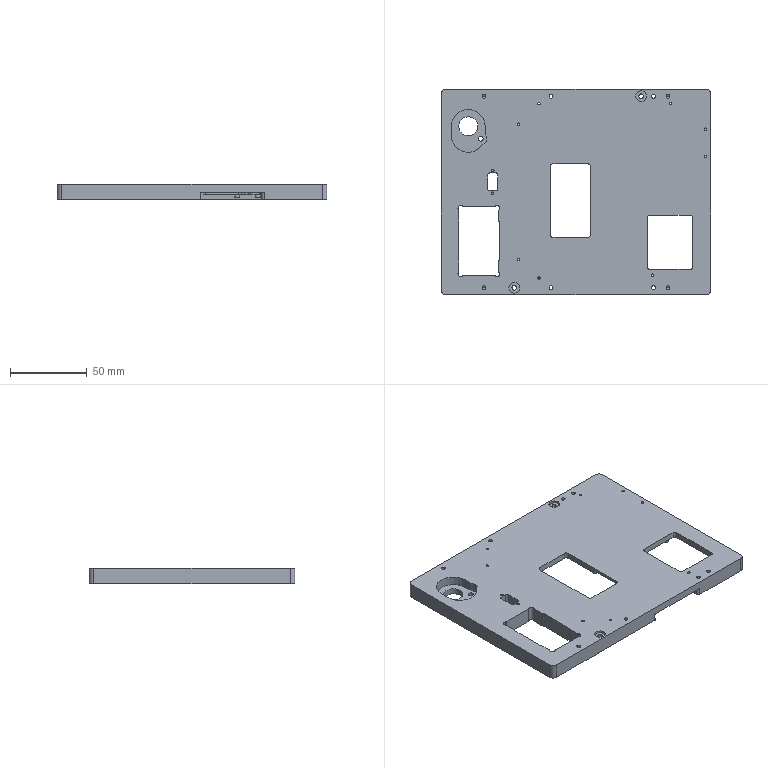NC program | NX | posted with a generic post | part box 176 x 134 x 10 mm
Lines 98 to 1138 of 17594:
(CAVITY_MILL , TOOL : D10)
N188 T04 M6
N190 G54
N192 G17 G0 G90 X-20.503 Y3.162 S9500 M3
N194 G43 Z30. H4
N196 Z1.5
N198 G94 G1 Y4.346 Z1.438 F1000.
N200 X-22.187 Y3.255 Z1.333
N202 X-22.361 Y3.15 Z1.322
N204 X-25.859 Y1.182 Z1.112
N206 X-26.039 Y1.088 Z1.101
N208 X-27.847 Y0.216 Z0.996
N210 X-26.039 Y-0.656 Z0.891
N212 X-22.187 Y-2.823 Z0.659
N214 X-20.503 Y-3.914 Z0.554
N216 Y4.346 Z0.121
N218 X-22.187 Y3.255 Z0.016
N220 X-22.361 Y3.15 Z0.005
N222 X-24.11 Y2.166 Z-0.1
N224 G2 X-27.847 Y0.216 R67.1 F3000.
N226 X-20.503 Y-3.914 R67.1
N228 G1 Y4.346
N230 G2 X-24.11 Y2.166 R67.1
N232 G1 X-26.316 Y6.088
N234 G2 X-32.497 Y3.047 R62.6
N236 G1 Y-2.614
N238 G2 X-17.697 Y-11.497 R62.6
N240 G1 X-16.003
N242 Y11.497
N244 X-18.239
N246 G2 X-26.316 Y6.088 R62.6
N248 G1 X-29.747 Y12.189
N250 G2 X-39.497 Y7.878 R55.6
N252 G1 Y-7.446
N254 G2 X-20.252 Y-18.497 R55.6
N256 G1 X-9.003
N258 Y18.497
N260 X-20.748
N262 G2 X-29.747 Y12.189 R55.6
N264 G1 X-33.179 Y18.291
N266 G2 X-46.497 Y13.2 R48.6
N268 G1 Y-12.768
N270 G2 X-22.998 Y-25.497 R48.6
N272 G1 X-2.003
N274 Y25.497
N276 X-23.444
N278 G2 X-33.179 Y18.291 R48.6
N280 G1 X-36.61 Y24.392
N282 G2 X-53.497 Y19.199 R41.6
N284 G1 Y-16.474
N286 G2 X-50.323 Y-19.158 R41.6
N288 X-25.986 Y-32.497 R41.6
N290 G1 X4.997
N292 Y32.497
N294 X-26.377
N296 G2 X-36.61 Y24.392 R41.6
N298 G1 X-40.042 Y30.493
N300 G2 X-57.003 Y26.051 R34.6
N302 G1 X-58.134
N304 G2 X-60.497 Y26.135 R33.1
N306 G1 Y-20.141
N308 G2 X-53.579 Y-25.788 R34.6
N310 X-29.294 Y-39.497 R34.6
N312 G1 X11.997
N314 Y39.497
N316 X-29.623
N318 G2 X-40.042 Y30.493 R34.6
N320 G1 X-43.473 Y36.594
N322 G2 X-57.003 Y33.051 R27.6
N324 G1 X-58.134
N326 G2 X-62.194 Y33.368 R26.1
N328 X-63.881 Y33.163 R27.6
N330 X-67.497 Y31.216 R27.6
N332 G1 Y-24.335
N334 G2 X-56.935 Y-32.619 R27.6
N336 X-33.055 Y-46.497 R27.6
N338 G1 X18.997
N340 Y46.497
N342 X-33.308
N344 G2 X-43.473 Y36.594 R27.6
N346 G1 X-46.904 Y42.695
N348 G2 X-57.003 Y40.051 R20.6
N350 G1 X-58.134
N352 G2 X-62.173 Y40.483 R19.1
N354 X-66.235 Y40.051 R20.6
N356 X-74.497 Y36.265 R20.6
N358 G1 Y-29.384
N360 G2 X-60.685 Y-39.619 R20.6
N362 G1 X-57.003
N364 G2 X-37.53 Y-53.497 R20.6
N366 G1 X25.997
N368 Y53.497
N370 X-37.685
N372 G2 X-46.904 Y42.695 R20.6
N374 G1 X-50.336 Y48.797
N376 G2 X-57.003 Y47.051 R13.6
N378 G1 X-58.134
N380 G2 X-62.128 Y47.729 R12.1
N382 X-66.37 Y47.051 R13.6
N384 G1 X-68.883
N386 G2 X-78.737 Y42.824 R13.6
N388 G1 X-81.497
N390 Y-35.943
N392 X-78.737
N394 G2 X-65.455 Y-46.619 R13.6
N396 G1 X-57.003
N398 G2 X-43.403 Y-60.219 R13.6
N400 G1 Y-60.497
N402 X32.997
N404 Y60.497
N406 X-43.404
N408 G2 X-50.336 Y48.797 R13.6
N410 G1 X-53.767 Y54.898
N412 G2 X-57.003 Y54.051 R6.6
N414 G1 X-58.134
N416 G2 X-61.941 Y55.757 R5.1
N418 X-66.37 Y54.051 R6.6
N420 G1 X-72.578
N422 G2 X-78.737 Y49.824 R6.6
N424 G1 X-86.5
N426 G2 X-92.997 Y55.262 R6.6
N428 G1 Y51.756
N430 G3 X-88.497 Y48.677 R8.
N432 G1 Y-41.796
N434 G3 X-92.997 Y-44.875 R8.
N436 G1 Y-48.38
N438 G2 X-86.5 Y-42.943 R6.6
N440 G1 X-78.737
N442 G2 X-72.137 Y-49.543 R6.6
N444 G1 Y-53.619
N446 X-57.003
N448 G2 X-50.403 Y-60.219 R6.6
N450 G1 Y-64.258
N452 G2 X-55.722 Y-71.997 R6.6
N454 G1 X-52.216
N456 G3 X-49.138 Y-67.497 R8.
N458 G1 X38.733
N460 G3 X41.811 Y-71.997 R8.
N462 G1 X45.316
N464 G2 X39.997 Y-64.258 R6.6
N466 G1 Y64.258
N468 G2 X45.316 Y71.997 R6.6
N470 G1 X41.811
N472 G3 X38.733 Y67.497 R8.
N474 G1 X-49.138
N476 G3 X-52.216 Y71.997 R8.
N478 G1 X-55.722
N480 G2 X-50.403 Y64.258 R6.6
N482 G1 Y60.576
N484 G2 X-53.767 Y54.898 R6.6
N486 G3 X-54.277 Y54.038 R1.
N488 G1 Z1.4
N490 G0 Z30.
N492 X-30.878 Y0.551
N494 Z1.4
N496 G1 X-34.997 Z1.184 F1000.
N498 Y-1.364 Z1.084
N500 X-33.137 Y-1.748 Z0.984
N502 X-28.184 Y-3.164 Z0.714
N504 X-26.402 Y-3.82 Z0.615
N506 X-24.62 Y-3.164 Z0.515
N508 X-21.303 Y-2.165 Z0.334
N510 X-19.454 Y-1.728 Z0.234
N512 Y0.551 Z0.115
N514 X-34.997 Z-0.7
N516 Y-0.406 Z-0.75
N518 Y-1.364 F3000.
N520 G2 X-26.402 Y-3.82 R60.1
N522 X-19.454 Y-1.728 R60.1
N524 G1 Y0.551
N526 X-34.997
N528 Y-0.406
N530 X-39.497
N532 Y-5.15
N534 G2 X-26.402 Y-8.642 R55.6
N536 X-14.954 Y-5.405 R55.6
N538 G1 Y5.051
N540 X-39.497
N542 Y-0.406
N544 X-46.497
N546 Y-11.623
N548 G2 X-26.402 Y-16.278 R48.6
N550 X-7.954 Y-11.674 R48.6
N552 G1 Y12.051
N554 X-46.497
N556 Y-0.406
N558 X-53.497
N560 Y-16.474
N562 G2 X-50.911 Y-18.619 R41.6
N564 G1 X-47.167
N566 G2 X-26.402 Y-24.172 R41.6
N568 X-5.63 Y-18.619 R41.6
N570 G1 X-0.954
N572 Y19.051
N574 X-53.497
N576 Y-0.406
N578 X-60.497
N580 Y-20.141
N582 G2 X-53.741 Y-25.619 R34.6
N584 G1 X-47.167
N586 G2 X-26.402 Y-32.542 R34.6
N588 X-5.631 Y-25.619 R34.6
N590 G1 X6.046
N592 Y26.051
N594 X-58.134
N596 G2 X-60.497 Y26.135 R33.1
N598 G1 Y-0.406
N600 X-67.497
N602 Y-24.335
N604 G2 X-56.935 Y-32.619 R27.6
N606 G1 X-47.167
N608 G2 X-26.402 Y-42.037 R27.6
N610 X-5.632 Y-32.619 R27.6
N612 G1 X13.046
N614 Y33.051
N616 X-58.134
N618 G2 X-62.194 Y33.368 R26.1
N620 X-63.881 Y33.163 R27.6
N622 X-67.497 Y31.216 R27.6
N624 G1 Y-0.406
N626 X-74.497
N628 Y-29.384
N630 G2 X-60.685 Y-39.619 R20.6
N632 G1 X-47.167
N634 G2 X-27.694 Y-53.497 R20.6
N636 G1 X-25.109
N638 G2 X-5.633 Y-39.619 R20.6
N640 G1 X20.046
N642 X20.045 Y39.689
N644 G2 X20.049 Y40.056 R20.6
N646 X19.588 Y40.051 R20.6
N648 G1 X-58.134
N650 G2 X-62.173 Y40.483 R19.1
N652 X-66.235 Y40.051 R20.6
N654 X-74.497 Y36.265 R20.6
N656 G1 Y-0.406
N658 X-81.497
N660 Y-35.943
N662 X-78.737
N664 G2 X-65.455 Y-46.619 R13.6
N666 G1 X-47.167
N668 G2 X-33.567 Y-60.219 R13.6
N670 G1 Y-60.497
N672 X-19.234
N674 G2 X-5.634 Y-46.619 R13.6
N676 G1 X20.441
N678 G2 X24.201 Y-47.149 R13.6
N680 X27.175 Y-46.641 R13.6
N682 X27.816 Y-44. R13.6
N684 X27.045 Y-39.488 R13.6
N686 G1 Y39.689
N688 G2 X27.834 Y44.253 R13.6
N690 X27.148 Y47.153 R13.6
N692 X24.201 Y47.857 R13.6
N694 X19.588 Y47.051 R13.6
N696 G1 X-58.134
N698 G2 X-62.128 Y47.729 R12.1
N700 X-66.37 Y47.051 R13.6
N702 G1 X-68.883
N704 G2 X-78.737 Y42.824 R13.6
N706 G1 X-81.497
N708 Y-0.406
N710 X-88.497
N712 Y-41.796
N714 G3 X-92.997 Y-44.875 R8.
N716 G1 Y-48.381
N718 G2 X-86.5 Y-42.943 R6.6
N720 G1 X-78.737
N722 G2 X-72.137 Y-49.543 R6.6
N724 G1 Y-53.619
N726 X-47.167
N728 G2 X-40.567 Y-60.219 R6.6
N730 G1 Y-65.5
N732 G2 X-46.005 Y-71.997 R6.6
N734 G1 X-42.499
N736 G3 X-39.42 Y-67.497 R8.
N738 G1 X-13.381
N740 G3 X-10.302 Y-71.997 R8.
N742 G1 X-6.796
N744 G2 X-12.234 Y-65.5 R6.6
N746 G1 Y-60.219
N748 G2 X-5.634 Y-53.619 R6.6
N750 G1 X20.441
N752 G2 X24.201 Y-54.794 R6.6
N754 X27.961 Y-53.619 R6.6
N756 G1 X34.045
N758 Y-48.512
N760 G2 X35.828 Y-44. R6.6
N762 X34.045 Y-39.488 R6.6
N764 G1 Y39.689
N766 G2 X35.878 Y44.253 R6.6
N768 X34.045 Y48.817 R6.6
N770 G1 Y54.051
N772 X28.814
N774 G2 X24.338 Y55.8 R6.6
N776 G1 X24.2 Y55.93
N778 G2 X19.588 Y54.051 R6.6
N780 G1 X-58.134
N782 G2 X-61.941 Y55.757 R5.1
N784 X-66.37 Y54.051 R6.6
N786 G1 X-72.578
N788 G2 X-78.737 Y49.824 R6.6
N790 G1 X-86.5
N792 G2 X-92.997 Y55.263 R6.6
N794 G1 Y51.756
N796 G3 X-88.497 Y48.677 R8.
N798 G1 Y-0.406
N800 G2 X-88.997 Y-1.273 R1.
N802 G1 X-94.997 Y-4.737
N804 Z0.75
N806 G0 Z30.
N808 X-30.878 Y0.551
N810 Z0.75
N812 G1 X-34.997 Z0.534 F1000.
N814 Y-1.364 Z0.434
N816 X-33.137 Y-1.748 Z0.334
N818 X-28.184 Y-3.164 Z0.064
N820 X-26.402 Y-3.82 Z-0.035
N822 X-24.62 Y-3.164 Z-0.135
N824 X-21.303 Y-2.165 Z-0.316
N826 X-19.454 Y-1.728 Z-0.416
N828 Y0.551 Z-0.535
N830 X-34.997 Z-1.35
N832 Y-0.406 Z-1.4
N834 Y-1.364 F3000.
N836 G2 X-26.402 Y-3.82 R60.1
N838 X-19.454 Y-1.728 R60.1
N840 G1 Y0.551
N842 X-34.997
N844 Y-0.406
N846 X-39.497
N848 Y-5.15
N850 G2 X-26.402 Y-8.642 R55.6
N852 X-14.954 Y-5.405 R55.6
N854 G1 Y5.051
N856 X-39.497
N858 Y-0.406
N860 X-46.497
N862 Y-11.623
N864 G2 X-26.402 Y-16.278 R48.6
N866 X-7.954 Y-11.674 R48.6
N868 G1 Y12.051
N870 X-46.497
N872 Y-0.406
N874 X-53.497
N876 Y-16.474
N878 G2 X-50.911 Y-18.619 R41.6
N880 G1 X-47.167
N882 G2 X-26.402 Y-24.172 R41.6
N884 X-5.631 Y-18.619 R41.6
N886 G1 X-0.954
N888 Y19.051
N890 X-53.497
N892 Y-0.406
N894 X-60.497
N896 Y-20.141
N898 G2 X-53.741 Y-25.619 R34.6
N900 G1 X-47.167
N902 G2 X-26.402 Y-32.542 R34.6
N904 X-5.631 Y-25.619 R34.6
N906 G1 X6.046
N908 Y26.051
N910 X-58.134
N912 G2 X-60.497 Y26.135 R33.1
N914 G1 Y-0.406
N916 X-67.497
N918 Y-24.335
N920 G2 X-56.935 Y-32.619 R27.6
N922 G1 X-47.167
N924 G2 X-26.402 Y-42.037 R27.6
N926 X-5.632 Y-32.619 R27.6
N928 G1 X13.046
N930 Y33.051
N932 X-58.134
N934 G2 X-62.194 Y33.368 R26.1
N936 X-63.881 Y33.163 R27.6
N938 X-67.497 Y31.216 R27.6
N940 G1 Y-0.406
N942 X-74.497
N944 Y-29.384
N946 G2 X-60.685 Y-39.619 R20.6
N948 G1 X-47.167
N950 G2 X-27.694 Y-53.497 R20.6
N952 G1 X-25.109
N954 G2 X-5.633 Y-39.619 R20.6
N956 G1 X20.046
N958 X20.045 Y39.689
N960 G2 X20.049 Y40.056 R20.6
N962 X19.588 Y40.051 R20.6
N964 G1 X-58.134
N966 G2 X-62.173 Y40.483 R19.1
N968 X-66.235 Y40.051 R20.6
N970 X-74.497 Y36.265 R20.6
N972 G1 Y-0.406
N974 X-81.497
N976 Y-35.943
N978 X-78.737
N980 G2 X-65.455 Y-46.619 R13.6
N982 G1 X-47.167
N984 G2 X-33.567 Y-60.219 R13.6
N986 G1 Y-60.497
N988 X-19.234
N990 G2 X-5.634 Y-46.619 R13.6
N992 G1 X20.441
N994 G2 X24.201 Y-47.149 R13.6
N996 X27.175 Y-46.641 R13.6
N998 X27.816 Y-44. R13.6
N1000 X27.045 Y-39.488 R13.6
N1002 G1 Y39.689
N1004 G2 X27.834 Y44.253 R13.6
N1006 X27.148 Y47.153 R13.6
N1008 X24.201 Y47.857 R13.6
N1010 X19.588 Y47.051 R13.6
N1012 G1 X-58.134
N1014 G2 X-62.128 Y47.729 R12.1
N1016 X-66.37 Y47.051 R13.6
N1018 G1 X-68.883
N1020 G2 X-78.737 Y42.824 R13.6
N1022 G1 X-81.497
N1024 Y-0.406
N1026 X-88.497
N1028 Y-41.796
N1030 G3 X-92.997 Y-44.875 R8.
N1032 G1 Y-48.382
N1034 G2 X-86.5 Y-42.943 R6.6
N1036 G1 X-78.737
N1038 G2 X-72.137 Y-49.543 R6.6
N1040 G1 Y-53.619
N1042 X-47.167
N1044 G2 X-40.567 Y-60.219 R6.6
N1046 G1 Y-65.5
N1048 G2 X-46.006 Y-71.997 R6.6
N1050 G1 X-42.499
N1052 G3 X-39.42 Y-67.497 R8.
N1054 G1 X-13.381
N1056 G3 X-10.302 Y-71.997 R8.
N1058 G1 X-6.795
N1060 G2 X-12.234 Y-65.5 R6.6
N1062 G1 Y-60.219
N1064 G2 X-5.634 Y-53.619 R6.6
N1066 G1 X20.441
N1068 G2 X24.201 Y-54.794 R6.6
N1070 X27.961 Y-53.619 R6.6
N1072 G1 X34.045
N1074 Y-48.512
N1076 G2 X35.828 Y-44. R6.6
N1078 X34.045 Y-39.488 R6.6
N1080 G1 Y39.689
N1082 G2 X35.878 Y44.253 R6.6
N1084 X34.045 Y48.817 R6.6
N1086 G1 Y54.051
N1088 X28.814
N1090 G2 X24.338 Y55.8 R6.6
N1092 G1 X24.2 Y55.93
N1094 G2 X19.588 Y54.051 R6.6
N1096 G1 X-58.134
N1098 G2 X-61.941 Y55.757 R5.1
N1100 X-66.37 Y54.051 R6.6
N1102 G1 X-72.578
N1104 G2 X-78.737 Y49.824 R6.6
N1106 G1 X-86.5
N1108 G2 X-92.997 Y55.264 R6.6
N1110 G1 Y51.756
N1112 G3 X-88.497 Y48.677 R8.
N1114 G1 Y-0.406
N1116 G2 X-88.997 Y-1.273 R1.
N1118 G1 X-94.997 Y-4.737
N1120 Z0.1
N1122 G0 Z30.
N1124 X-24.7 Y-1.606
N1126 Z0.1
N1128 G1 X-24.433 Y-0.962 Z0.063 F1000.
N1130 X-22.568 Y2.7 Z-0.152
N1132 X-20.395 Y6.188 Z-0.367
N1134 X-19.39 Y7.551 Z-0.456
N1136 X-23.62 Z-0.678
N1138 X-23.846 Y6.485 Z-0.735
N1140 X-24.805 Y3.754 Z-0.886
N1142 X-26.151 Y1.191 Z-1.038
N1144 X-27.403 Y-0.592 Z-1.152
N1146 X-28.217 Y-1.56 Z-1.219
N1148 X-28.988 Y-2.33 Z-1.276
N1150 X-27.298 Y-2.345 Z-1.364
N1152 X-26.764 Y-2.372 Z-1.392
N1154 X-25.081 Y-2.526 Z-1.481
N1156 X-24.433 Y-0.962 Z-1.57
N1158 X-22.568 Y2.7 Z-1.785
N1160 X-20.395 Y6.188 Z-2.
N1162 X-19.39 Y7.551 Z-2.089
N1164 X-21.505 Z-2.2
N1166 X-23.62 F3000.
N1168 G2 X-28.988 Y-2.33 R19.76
N1170 X-25.081 Y-2.526 R47.61
N1172 X-19.39 Y7.551 R47.76
N1174 G1 X-21.505
N1176 Y12.051
N1178 X-27.695
N1180 G2 X-46.497 Y-3.188 R15.26
N1182 G1 Y-10.352
N1184 G2 X-22.105 Y-7.454 R43.11
N1186 X-9.102 Y12.051 R43.26
N1188 G1 X-21.505
N1190 Y19.051
N1192 X-39.273
N1194 G2 X-46.626 Y19.051 R-8.26
N1196 G1 X-46.003 Y17.797
N1198 G2 X-36.806 Y14.707 R6.86
N1200 X-46.003 Y17.797 R-6.86
N1202 G1 X-46.626 Y19.051
N1204 X-53.497
N1206 Y-16.474
N1208 G2 X-50.911 Y-18.619 R41.6
N1210 G1 X-47.4
N1212 G2 X-16.905 Y-16.068 R36.11
N1214 X-0.955 Y9.445 R36.26
N1216 G1 Y19.051
N1218 X-21.505
N1220 Y26.051
N1222 X-60.497
N1224 Y-20.14
N1226 G2 X-53.741 Y-25.619 R34.6
N1228 G1 X-47.167
N1230 G2 X-45.487 Y-25.659 R34.6
N1232 X-13.719 Y-25.43 R29.11
N1234 X-10.153 Y-22.715 R34.71
N1236 X6.045 Y5.413 R29.26
N1238 G1 Y26.051
N1240 X-21.505
N1242 Y33.051
N1244 X-60.76
N1246 G2 X-61.81 Y33.071 R27.6
N1248 X-62.86 Y33.051 R27.6
N1250 G1 X-64.058
N1252 G2 X-67.497 Y31.216 R27.6
N1254 G1 Y-24.335
N1256 G2 X-56.935 Y-32.619 R27.6
N1258 G1 X-47.167
N1260 G2 X-43.477 Y-32.866 R27.6
N1262 X-14.141 Y-33.962 R22.11
N1264 X-11.734 Y-33.301 R27.6
N1266 X-2.49 Y-26.437 R27.71
N1268 X13.045 Y0.635 R22.26
N1270 G1 Y33.051
N1272 X-21.505
N1274 Y40.051
N1276 X-60.76
N1278 G2 X-61.81 Y40.077 R20.6
N1280 X-62.86 Y40.051 R20.6
N1282 G1 X-66.236
N1284 G2 X-74.497 Y36.265 R20.6
N1286 G1 Y-29.384
N1288 G2 X-60.685 Y-39.619 R20.6
N1290 G1 X-47.167
N1292 G2 X-41.222 Y-40.495 R20.6
N1294 X-16.241 Y-42.559 R15.11
N1296 X-7.913 Y-39.745 R20.6
N1298 X7.665 Y-30.968 R20.71
N1300 G1 X12.478 Y-32.321
N1302 G3 X22.045 Y-33.717 R13.26
N1304 G1 Y-38.175
N1306 G3 X12.148 Y-33.181 R18.71
N1308 X12.478 Y-32.321 R5.
N1310 G1 X7.665 Y-30.968
N1312 G2 X20.045 Y-5.574 R15.26
N1314 G1 Y40.051
N1316 X-21.505
N1318 Y47.051
N1320 X-60.76
N1322 G2 X-61.81 Y47.091 R13.6
N1324 X-62.86 Y47.051 R13.6
N1326 G1 X-68.883
N1328 G2 X-78.737 Y42.824 R13.6
N1330 G1 X-81.497
N1332 Y-35.943
N1334 X-78.737
N1336 G2 X-65.455 Y-46.619 R13.6
N1338 G1 X-47.167
N1340 G2 X-37.506 Y-50.647 R13.6
N1342 X-34.059 Y-56.595 R-8.11
N1344 G1 X-33.259 Y-55.446
N1346 G2 X-34.934 Y-46.105 R6.71
N1348 X-33.259 Y-55.446 R-6.71
N1350 G1 X-34.059 Y-56.595
N1352 G2 X-33.567 Y-60.219 R13.6
N1354 G1 Y-60.497
N1356 X-19.234
N1358 G2 X-15.251 Y-50.602 R13.6
N1360 X-5.634 Y-46.619 R13.6
N1362 G1 X-3.714
N1364 G2 X21.807 Y-46.619 R13.71
N1366 G1 X27.045
N1368 Y-22.853
N1370 G2 X27.045 Y-18.749 R-8.26
N1372 G1 X25.689 Y-19.097
N1374 G2 X20.749 Y-27.446 R6.86
N1376 X25.689 Y-19.097 R-6.86
N1378 G1 X27.045 Y-18.749
N1380 Y47.051
N1382 X25.464
N1384 G2 X24.201 Y47.109 R13.6
N1386 X22.938 Y47.051 R13.6
N1388 G1 X-21.505
N1390 Y54.051
N1392 X-60.76
N1394 G2 X-61.81 Y54.135 R6.6
N1396 X-62.86 Y54.051 R6.6
N1398 G1 X-72.578
N1400 G2 X-78.737 Y49.824 R6.6
N1402 G1 X-86.5
N1404 G2 X-92.997 Y55.265 R6.6
N1406 G1 Y51.757
N1408 G3 X-88.497 Y48.677 R8.
N1410 G1 Y-41.796
N1412 G3 X-92.997 Y-44.875 R8.
N1414 G1 Y-48.384
N1416 G2 X-86.5 Y-42.943 R6.6
N1418 G1 X-78.737
N1420 G2 X-72.137 Y-49.543 R6.6
N1422 G1 Y-53.619
N1424 X-47.167
N1426 G2 X-40.567 Y-60.219 R6.6
N1428 G1 Y-65.5
N1430 G2 X-46.007 Y-71.997 R6.6
N1432 G1 X-42.499
N1434 G3 X-39.42 Y-67.497 R8.
N1436 G1 X-13.381
N1438 G3 X-10.301 Y-71.997 R8.
N1440 G1 X-6.794
N1442 G2 X-12.234 Y-65.5 R6.6
N1444 G1 Y-60.219
N1446 G2 X-5.634 Y-53.619 R6.6
N1448 G1 X1.183
N1450 X2.637
N1452 G2 X15.455 Y-53.619 R-6.71
N1454 G1 X16.909
N1456 X34.045
N1458 Y54.051
N1460 X25.464
N1462 G2 X24.201 Y54.173 R6.6
N1464 X22.938 Y54.051 R6.6
N1466 G1 X-21.505
N1468 G3 X-22.371 Y53.551 R1.
N1470 G1 Z-0.7
N1472 G0 X-24.7 Y-1.606
N1474 G1 X-24.433 Y-0.962 Z-0.737 F1000.
N1476 X-22.568 Y2.7 Z-0.952
N1478 X-20.395 Y6.188 Z-1.167
N1480 X-19.39 Y7.551 Z-1.256
N1482 X-23.62 Z-1.478
N1484 X-23.846 Y6.485 Z-1.535
N1486 X-24.805 Y3.754 Z-1.686
N1488 X-26.151 Y1.191 Z-1.838
N1490 X-27.403 Y-0.592 Z-1.952
N1492 X-28.217 Y-1.56 Z-2.019
N1494 X-28.988 Y-2.33 Z-2.076
N1496 X-27.298 Y-2.345 Z-2.164
N1498 X-26.764 Y-2.372 Z-2.192
N1500 X-25.081 Y-2.526 Z-2.281
N1502 X-24.433 Y-0.962 Z-2.37
N1504 X-22.568 Y2.7 Z-2.585
N1506 X-20.395 Y6.188 Z-2.8
N1508 X-19.39 Y7.551 Z-2.889
N1510 X-21.505 Z-3.
N1512 X-23.62 F3000.
N1514 G2 X-28.988 Y-2.33 R19.76
N1516 X-25.081 Y-2.526 R47.61
N1518 X-19.39 Y7.551 R47.76
N1520 G1 X-21.505
N1522 Y12.051
N1524 X-27.695
N1526 G2 X-46.498 Y-3.188 R15.26
N1528 G1 Y-10.352
N1530 G2 X-22.105 Y-7.454 R43.11
N1532 X-9.102 Y12.051 R43.26
N1534 G1 X-21.505
N1536 Y19.051
N1538 X-39.273
N1540 G2 X-46.626 Y19.051 R-8.26
N1542 G1 X-46.003 Y17.797
N1544 G2 X-36.806 Y14.707 R6.86
N1546 X-46.003 Y17.797 R-6.86
N1548 G1 X-46.626 Y19.051
N1550 X-53.498
N1552 Y-16.474
N1554 G2 X-50.911 Y-18.619 R41.6
N1556 G1 X-47.4
N1558 G2 X-16.905 Y-16.068 R36.11
N1560 X-0.955 Y9.445 R36.26
N1562 G1 Y19.051
N1564 X-21.505
N1566 Y26.051
N1568 X-60.498
N1570 Y-20.14
N1572 G2 X-53.741 Y-25.619 R34.6
N1574 G1 X-47.167
N1576 G2 X-45.487 Y-25.659 R34.6
N1578 X-13.719 Y-25.43 R29.11
N1580 X-10.153 Y-22.715 R34.71
N1582 X6.045 Y5.413 R29.26
N1584 G1 Y26.051
N1586 X-21.505
N1588 Y33.051
N1590 X-60.76
N1592 G2 X-61.81 Y33.071 R27.6
N1594 X-62.86 Y33.051 R27.6
N1596 G1 X-64.058
N1598 G2 X-67.498 Y31.216 R27.6
N1600 G1 Y-24.335
N1602 G2 X-56.935 Y-32.619 R27.6
N1604 G1 X-47.167
N1606 G2 X-43.477 Y-32.866 R27.6
N1608 X-14.142 Y-33.962 R22.11
N1610 X-11.734 Y-33.3 R27.6
N1612 X-2.49 Y-26.437 R27.71
N1614 X13.045 Y0.635 R22.26
N1616 G1 Y33.051
N1618 X-21.505
N1620 Y40.051
N1622 X-60.76
N1624 G2 X-61.81 Y40.077 R20.6
N1626 X-62.86 Y40.051 R20.6
N1628 G1 X-66.236
N1630 G2 X-74.498 Y36.265 R20.6
N1632 G1 Y-29.384
N1634 G2 X-60.685 Y-39.619 R20.6
N1636 G1 X-47.167
N1638 G2 X-41.222 Y-40.495 R20.6
N1640 X-16.241 Y-42.558 R15.11
N1642 X-7.913 Y-39.745 R20.6
N1644 X7.665 Y-30.968 R20.71
N1646 G1 X12.478 Y-32.321
N1648 G3 X22.045 Y-33.717 R13.26
N1650 G1 Y-38.175
N1652 G3 X12.148 Y-33.181 R18.71
N1654 X12.478 Y-32.321 R5.
N1656 G1 X7.665 Y-30.968
N1658 G2 X20.045 Y-5.574 R15.26
N1660 G1 Y40.051
N1662 X-21.505
N1664 Y47.051
N1666 X-60.76
N1668 G2 X-61.81 Y47.091 R13.6
N1670 X-62.86 Y47.051 R13.6
N1672 G1 X-68.883
N1674 G2 X-78.737 Y42.824 R13.6
N1676 G1 X-81.498
N1678 Y-35.943
N1680 X-78.737
N1682 G2 X-65.455 Y-46.619 R13.6
N1684 G1 X-47.167
N1686 G2 X-37.506 Y-50.647 R13.6
N1688 X-34.059 Y-56.595 R-8.11
N1690 G1 X-33.259 Y-55.446
N1692 G2 X-34.934 Y-46.105 R6.71
N1694 X-33.259 Y-55.446 R-6.71
N1696 G1 X-34.059 Y-56.595
N1698 G2 X-33.567 Y-60.219 R13.6
N1700 G1 Y-60.498
N1702 X-19.234
N1704 G2 X-5.634 Y-46.619 R13.6
N1706 G1 X-3.714
N1708 G2 X21.807 Y-46.619 R13.71
N1710 G1 X27.045
N1712 Y-22.853
N1714 G2 X27.045 Y-18.749 R-8.26
N1716 G1 X25.689 Y-19.097
N1718 G2 X20.749 Y-27.446 R6.86
N1720 X25.689 Y-19.097 R-6.86
N1722 G1 X27.045 Y-18.749
N1724 Y47.051
N1726 X25.464
N1728 G2 X24.201 Y47.109 R13.6
N1730 X22.938 Y47.051 R13.6
N1732 G1 X-21.505
N1734 Y54.051
N1736 X-60.76
N1738 G2 X-61.81 Y54.135 R6.6
N1740 X-62.86 Y54.051 R6.6
N1742 G1 X-72.578
N1744 G2 X-78.737 Y49.824 R6.6
N1746 G1 X-86.5
N1748 G2 X-92.998 Y55.266 R6.6
N1750 G1 Y51.757
N1752 G3 X-88.498 Y48.677 R8.
N1754 G1 Y-41.796
N1756 G3 X-92.998 Y-44.876 R8.
N1758 G1 Y-48.385
N1760 G2 X-86.5 Y-42.943 R6.6
N1762 G1 X-78.737
N1764 G2 X-72.137 Y-49.543 R6.6
N1766 G1 Y-53.619
N1768 X-47.167
N1770 G2 X-40.567 Y-60.219 R6.6
N1772 G1 Y-65.5
N1774 G2 X-46.008 Y-71.998 R6.6
N1776 G1 X-42.5
N1778 G3 X-39.42 Y-67.498 R8.
N1780 G1 X-13.381
N1782 G3 X-10.301 Y-71.998 R8.
N1784 G1 X-6.793
N1786 G2 X-12.234 Y-65.5 R6.6
N1788 G1 Y-60.219
N1790 G2 X-5.634 Y-53.619 R6.6
N1792 G1 X2.637
N1794 G2 X15.455 Y-53.619 R-6.71
N1796 G1 X34.045
N1798 Y54.051
N1800 X25.464
N1802 G2 X24.201 Y54.173 R6.6
N1804 X22.938 Y54.051 R6.6
N1806 G1 X-21.505
N1808 G3 X-22.371 Y53.551 R1.
N1810 G1 Z-1.5
N1812 G0 X11.8 Y5.691
N1814 G1 X14.325 Y6.262 Z-1.636 F1000.
N1816 X15.545 Y6.396 Z-1.7
N1818 Y9.837 Z-1.88
N1820 X7.094 Z-2.323
N1822 Y3.911 Z-2.634
N1824 X8.192 Y4.458 Z-2.698
N1826 X11.201 Y5.556 Z-2.866
N1828 X14.325 Y6.262 Z-3.034
N1830 X15.545 Y6.396 Z-3.098
N1832 Y9.837 Z-3.279
N1834 X11.32 Z-3.5
N1836 X7.094 F3000.
N1838 Y3.911
N1840 G2 X15.545 Y6.396 R25.1
N1842 G1 Y9.837
N1844 X11.32
N1846 Y14.337
N1848 X2.438
N1850 G2 X2.594 Y11.796 R20.85
N1852 G1 Y-5.214
N1854 X1.706 Y-10.135
N1856 G3 X-0.308 Y-18.553 R18.6
N1858 G1 Y-19.844
N1860 X-3.091 Y-20.6
N1862 X-5.703
N1864 G3 X0.345 Y-9.68 R18.6
N1866 X1.706 Y-10.135 R5.
N1868 G1 X2.594 Y-5.214
N1870 G2 X18.292 Y2.047 R20.6
N1872 G1 X20.045
N1874 Y14.337
N1876 X11.32
N1878 Y21.337
N1880 X-3.817
N1882 G2 X-9.672 Y22.661 R13.6
N1884 X-4.406 Y11.795 R13.85
N1886 G1 Y-6.65
N1888 G2 X-18.006 Y-20.25 R13.6
N1890 G1 X-24.463
N1892 Y-28.41
N1894 G2 X-25.2 Y-32.867 R13.85
N1896 X-13.015 Y-25.6 R13.85
N1898 G1 X-2.424
N1900 X4.692 Y-23.666
N1902 Y-18.553
N1904 G2 X18.292 Y-4.953 R13.6
N1906 G1 X21.966
N1908 G2 X27.045 Y-5.918 R13.85
N1910 G1 Y21.337
N1912 X11.32
N1914 Y28.337
N1916 X-3.817
N1918 G2 X-10.417 Y34.937 R6.6
N1920 G1 Y49.848
N1922 X-35.57
N1924 Y32.991
N1926 G2 X-42.42 Y26.141 R6.85
N1928 G1 X-60.196
N1930 G2 X-65.341 Y23.676 R6.6
N1932 G1 X-72.304
N1934 G2 X-78.904 Y30.276 R6.6
N1936 G1 Y49.824
N1938 X-86.5
N1940 G2 X-92.998 Y55.267 R6.6
N1942 G1 Y51.757
N1944 G3 X-88.498 Y48.677 R8.
N1946 G1 Y-41.796
N1948 G3 X-92.998 Y-44.876 R8.
N1950 G1 Y-48.386
N1952 G2 X-86.5 Y-42.943 R6.6
N1954 G1 X-77.637
N1956 G2 X-72.461 Y-45.449 R6.6
N1958 G1 X-51.466
N1960 Y-25.678
N1962 X-65.466
N1964 G2 X-71.072 Y-26.805 R14.5
N1966 G1 X-71.886
N1968 G2 X-74.498 Y-26.568 R14.5
N1970 G1 Y-29.183
N1972 G2 X-67.79 Y-31.449 R20.6
N1974 G1 X-65.466
N1976 Y-25.678
N1978 X-58.466
N1980 Y-21.684
N1982 G2 X-63.956 Y-14.672 R13.85
N1984 G1 X-63.149 Y-6.758
N1986 X-63.956 Y-14.672
N1988 G2 X-71.072 Y-19.805 R7.5
N1990 G1 X-71.886
N1992 G2 X-79.386 Y-12.305 R7.5
N1994 G1 Y-3.048
N1996 G2 X-71.886 Y4.452 R7.5
N1998 G1 X-71.072
N2000 G2 X-64.735 Y0.962 R7.5
N2002 G1 X-65.918 Y0.214
N2004 G2 X-64.972 Y-3.048 R6.1
N2006 G1 Y-12.305
N2008 G2 X-71.072 Y-18.405 R6.1
N2010 G1 X-71.886
N2012 G2 X-77.986 Y-12.305 R6.1
N2014 G1 Y-3.048
N2016 G2 X-71.886 Y3.052 R6.1
N2018 G1 X-71.072
N2020 G2 X-65.918 Y0.214 R6.1
N2022 G1 X-64.735 Y0.962
N2024 Y11.793
N2026 G2 X-63.812 Y16.762 R13.85
N2028 G1 X-59.401 Y20.186
N2030 X-63.812 Y16.762
N2032 G2 X-65.341 Y16.676 R13.6
N2034 G1 X-72.304
N2036 G2 X-75.37 Y17.026 R13.6
N2038 G1 X-73.377 Y10.503
N2040 X-75.37 Y17.026
N2042 G2 X-81.498 Y20.254 R13.6
N2044 G1 X-83.241 Y25.693
N2046 X-81.498 Y20.254
N2048 Y-35.943
N2050 X-77.637
N2052 G2 X-69.771 Y-38.449 R13.6
N2054 G1 X-58.466
N2056 Y-25.678
N2058 X-51.466
N2060 Y-18.553
N2062 G2 X-51.264 Y-16.933 R6.6
N2064 X-57.735 Y-10.094 R6.85
N2066 G1 Y11.793
N2068 G2 X-50.885 Y18.643 R6.85
N2070 G1 X-21.271
N2072 Y30.143
N2074 G2 X-21.917 Y34.937 R18.1
N2076 G1 Y38.348
N2078 X-24.07
N2080 Y32.991
N2082 G2 X-24.292 Y30.143 R18.35
N2084 G1 X-21.271
N2086 Y25.643
N2088 X-18.256
N2090 G2 X-12.269 Y24.281 R13.85
N2092 X-17.417 Y34.937 R13.6
N2094 G1 Y42.848
N2096 X-28.57
N2098 Y32.991
N2100 G2 X-30.68 Y25.643 R13.85
N2102 G1 X-21.271
N2104 Y18.643
N2106 X-18.256
N2108 G2 X-11.406 Y11.793 R6.85
N2110 G1 Y-6.65
N2112 G2 X-18.006 Y-13.25 R6.6
N2114 G1 X-32.397
N2116 G2 X-37.497 Y-8.15 R5.1
N2118 G1 Y-6.918
N2120 X-42.32
N2122 Y-11.953
N2124 X-38.063
N2126 G2 X-31.463 Y-18.553 R6.6
N2128 G1 Y-28.41
N2130 G2 X-32.287 Y-31.666 R6.85
N2132 G1 X-26.128 Y-34.993
N2134 G2 X-26.238 Y-35.192 R13.85
N2136 G1 X-26.194
N2138 G2 X-26.128 Y-34.993 R13.85
N2140 G1 X-32.287 Y-31.666
N2142 G2 X-38.313 Y-35.26 R6.85
N2144 G1 X-40.79
N2146 Y-44.056
N2148 G2 X-39.229 Y-48.319 R6.6
N2150 G1 Y-52.204
N2152 G2 X-40.567 Y-56.188 R6.6
N2154 G1 Y-65.5
N2156 G2 X-46.009 Y-71.998 R6.6
N2158 G1 X-42.5
N2160 G3 X-39.42 Y-67.498 R8.
N2162 G1 X-13.381
N2164 G3 X-10.301 Y-71.998 R8.
N2166 G1 X-6.792
N2168 G2 X-12.234 Y-65.5 R6.6
N2170 G1 Y-58.182
N2172 X-30.559
N2174 G2 X-33.408 Y-57.536 R6.6
N2176 G1 X-35.215 Y-62.35
N2178 X-33.408 Y-57.536
N2180 G2 X-37.159 Y-51.582 R6.6
N2182 G1 Y-48.792
N2184 G2 X-30.559 Y-42.192 R6.6
N2186 G1 X-19.865
N2188 Y-39.45
N2190 G2 X-13.015 Y-32.6 R6.85
N2192 G1 X-1.489
N2194 X11.692 Y-29.016
N2196 Y-18.553
N2198 G2 X18.292 Y-11.953 R6.6
N2200 G1 X21.966
N2202 G2 X26.479 Y-13.65 R6.85
N2204 G1 X29.605 Y-16.387
N2206 X34.045
N2208 Y28.337
N2210 X11.32
N2212 G3 X10.453 Y27.837 R1.
N2214 G1 Z-2.
N2216 G0 X7.094 Y8.407
N2218 G1 Y3.911 Z-2.236 F1000.
N2220 X8.192 Y4.458 Z-2.3
N2222 X11.201 Y5.556 Z-2.468
N2224 X14.325 Y6.262 Z-2.636
N2226 X15.545 Y6.396 Z-2.7
N2228 Y9.837 Z-2.88
N2230 X7.094 Z-3.323
N2232 Y3.911 Z-3.634
N2234 X8.192 Y4.458 Z-3.698
N2236 X11.201 Y5.556 Z-3.866
N2238 X14.325 Y6.262 Z-4.034
N2240 X15.545 Y6.396 Z-4.098
N2242 Y9.837 Z-4.279
N2244 X11.32 Z-4.5
N2246 X7.094 F3000.
N2248 Y3.911
N2250 G2 X15.545 Y6.396 R25.1
N2252 G1 Y9.837
N2254 X11.32
N2256 Y14.337
N2258 X2.438
N2260 G2 X2.594 Y11.793 R20.85
N2262 G1 Y-5.214